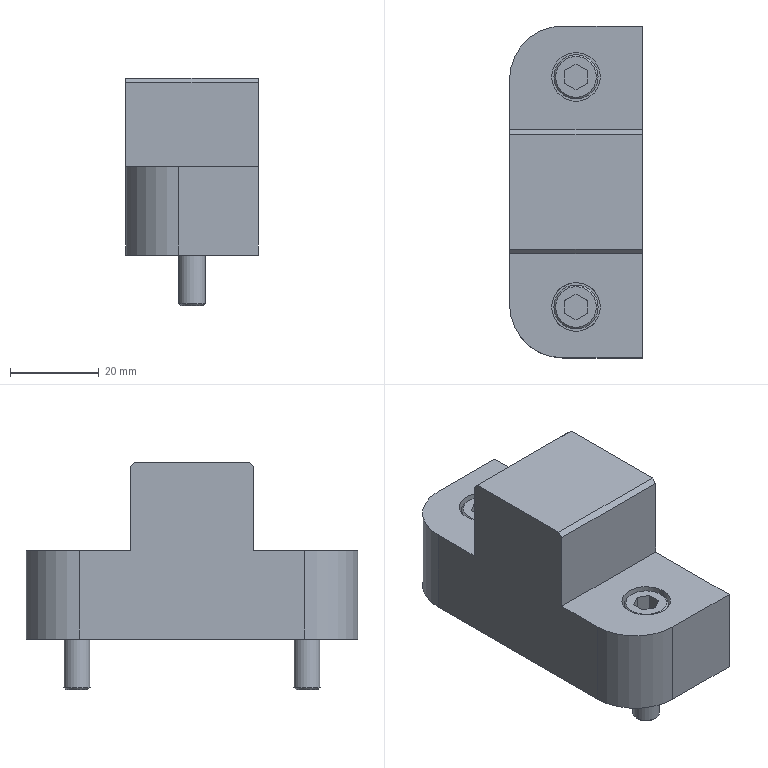Part | STEP file | LKM-Top Locks-TOP_75-B | 3 solids | 50 faces | box 30 x 75 x 51.5 mm | volume 60575 mm3 | plane 34 | cylinder 12 | cone 4 | commonest cylinder face diameters 6.5 x3 11 x3 6 x2 10 x2 24 x2